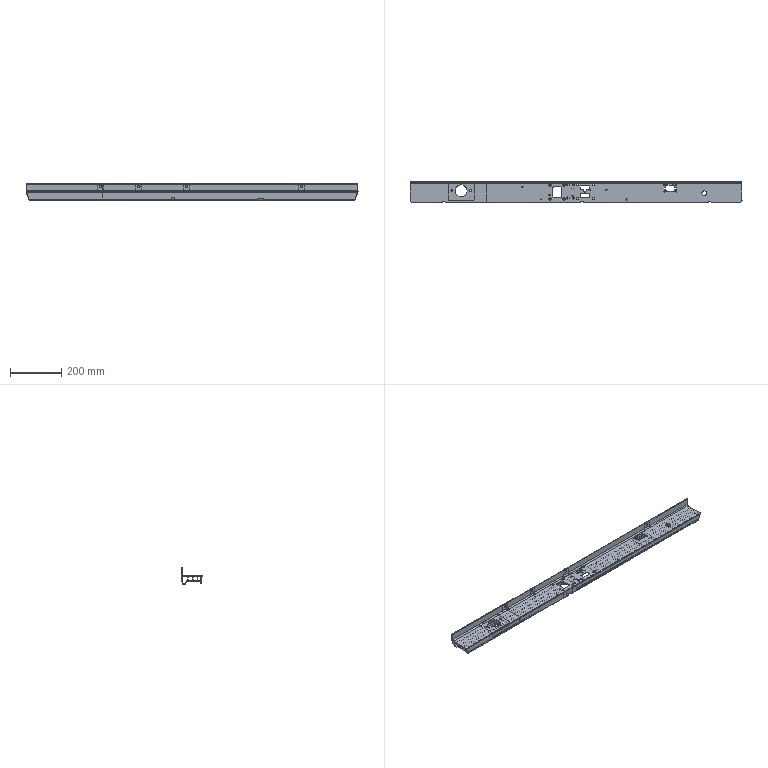Part | 3 solids | 645 faces | box 1301 x 81.1 x 63 mm | volume 821893 mm3 | plane 325 | cylinder 318 | spline 2 | commonest cylinder face diameters 4 x72 1 x58 2 x49 10 x43 7 x20 6.5 x15